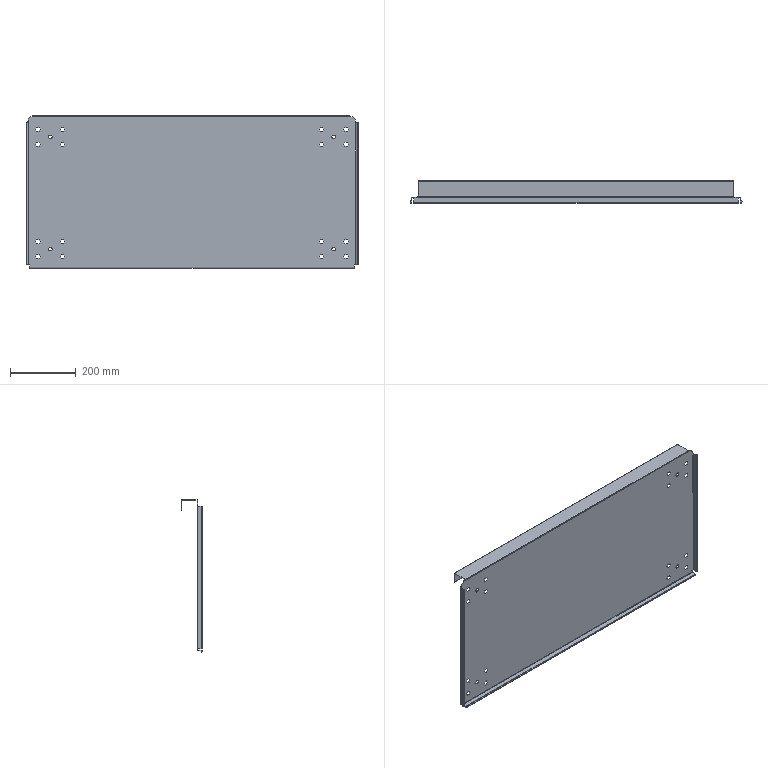Part | SolidWorks | features ICE 18, EdgeFlange 8, FlatPattern 1, HoleWzd 1, SMBaseFlange 1, SheetMetal 1 | 1 solid | 182 faces | box 1007 x 66.2 x 462.805 mm | volume 687365 mm3 | plane 154 | cylinder 26 | spline 2 | commonest cylinder face diameters 11 x8 1 x5 3.4 x5 2 x3 4.4 x3 40 x2